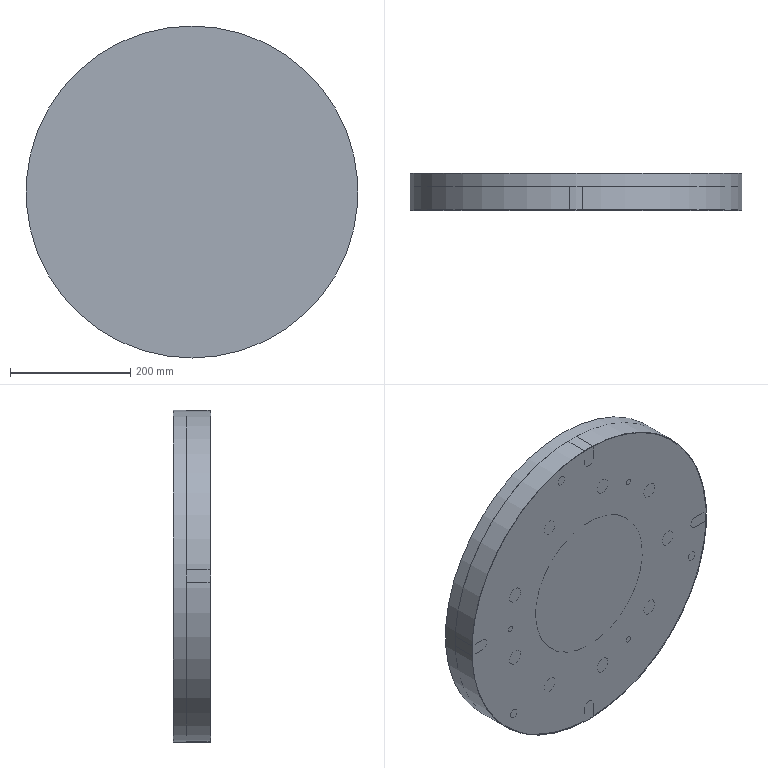NC program | NX | posted with a generic post | part box 552 x 62 x 552 mm
Whole program:
N10 G17 G21 G94 G90
(CAVITY_MILL_1 , TOOL : D8)
N12 T03 M6
N14 G54
N16 G17 G0 G90 X136.011 Y-125.254 S900 M3
N18 G43 Z19. H3
N20 Z-6.5
N22 G94 G1 X136.461 Y-125.633 Z-6.521 F80.
N24 X137.059 Y-126.025 Z-6.546
N26 X147.91 Y-113.092 Z-7.135
N28 X147.421 Y-112.572 Z-7.16
N30 X146.976 Y-112.198 Z-7.18
N32 X146.378 Y-111.807 Z-7.205
N34 X140.952 Y-118.273 Z-7.5
N36 X135.526 Y-124.739
N38 G3 X137.059 Y-126.025 R8.5
N40 G1 X147.91 Y-113.092
N42 G3 X146.378 Y-111.807 R8.49
N44 G1 X140.952 Y-118.273
N46 G3 X141.014 Y-118.977 R0.5
N48 X141.718 Y-118.916 R0.5
N50 G1 Z-7.3
N52 G0 Z-6.7
N54 X136.011 Y-125.254
N56 Z-7.
N58 G1 X136.461 Y-125.633 Z-7.021
N60 X137.059 Y-126.025 Z-7.046
N62 X147.91 Y-113.092 Z-7.635
N64 X147.421 Y-112.572 Z-7.66
N66 X146.976 Y-112.198 Z-7.68
N68 X146.378 Y-111.807 Z-7.705
N70 X140.952 Y-118.273 Z-8.
N72 X135.526 Y-124.739
N74 G3 X137.059 Y-126.025 R8.5
N76 G1 X147.91 Y-113.092
N78 G3 X146.378 Y-111.807 R8.49
N80 G1 X140.952 Y-118.273
N82 G3 X141.014 Y-118.977 R0.5
N84 X141.718 Y-118.916 R0.5
N86 G1 Z-7.8
N88 G0 Z-6.7
N90 X136.011 Y-125.254
N92 Z-7.5
N94 G1 X136.461 Y-125.633 Z-7.521
N96 X137.059 Y-126.025 Z-7.546
N98 X147.91 Y-113.092 Z-8.135
N100 X147.421 Y-112.572 Z-8.16
N102 X146.976 Y-112.198 Z-8.18
N104 X146.378 Y-111.807 Z-8.205
N106 X140.952 Y-118.273 Z-8.5
N108 X135.526 Y-124.739
N110 G3 X137.059 Y-126.025 R8.5
N112 G1 X147.91 Y-113.092
N114 G3 X146.378 Y-111.807 R8.49
N116 G1 X140.952 Y-118.273
N118 G3 X141.014 Y-118.977 R0.5
N120 X141.718 Y-118.916 R0.5
N122 G1 Z-8.3
N124 G0 Z-6.7
N126 X136.011 Y-125.254
N128 Z-8.
N130 G1 X136.461 Y-125.633 Z-8.021
N132 X137.059 Y-126.025 Z-8.046
N134 X147.91 Y-113.092 Z-8.635
N136 X147.421 Y-112.572 Z-8.66
N138 X146.976 Y-112.198 Z-8.68
N140 X146.378 Y-111.807 Z-8.705
N142 X140.952 Y-118.273 Z-9.
N144 X135.526 Y-124.739
N146 G3 X137.059 Y-126.025 R8.5
N148 G1 X147.91 Y-113.092
N150 G3 X146.378 Y-111.807 R8.49
N152 G1 X140.952 Y-118.273
N154 G3 X141.014 Y-118.977 R0.5
N156 X141.718 Y-118.916 R0.5
N158 G1 Z-8.8
N160 G0 Z-6.7
N162 X136.011 Y-125.254
N164 Z-8.5
N166 G1 X136.461 Y-125.633 Z-8.521
N168 X137.059 Y-126.025 Z-8.546
N170 X147.91 Y-113.092 Z-9.135
N172 X147.421 Y-112.572 Z-9.16
N174 X146.976 Y-112.198 Z-9.18
N176 X146.378 Y-111.807 Z-9.205
N178 X140.952 Y-118.273 Z-9.5
N180 X135.526 Y-124.739
N182 G3 X137.059 Y-126.025 R8.5
N184 G1 X147.91 Y-113.092
N186 G3 X146.378 Y-111.807 R8.49
N188 G1 X140.952 Y-118.273
N190 G3 X141.014 Y-118.977 R0.5
N192 X141.718 Y-118.916 R0.5
N194 G1 Z-9.3
N196 G0 Z-6.7
N198 X136.011 Y-125.254
N200 Z-9.
N202 G1 X136.461 Y-125.633 Z-9.021
N204 X137.059 Y-126.025 Z-9.046
N206 X147.91 Y-113.092 Z-9.635
N208 X147.421 Y-112.572 Z-9.66
N210 X146.976 Y-112.198 Z-9.68
N212 X146.378 Y-111.807 Z-9.705
N214 X140.952 Y-118.273 Z-10.
N216 X135.526 Y-124.739
N218 G3 X137.059 Y-126.025 R8.5
N220 G1 X147.91 Y-113.092
N222 G3 X146.378 Y-111.807 R8.49
N224 G1 X140.952 Y-118.273
N226 G3 X141.014 Y-118.977 R0.5
N228 X141.718 Y-118.916 R0.5
N230 G1 Z-9.8
N232 G0 Z-6.7
N234 X136.011 Y-125.254
N236 Z-9.5
N238 G1 X136.461 Y-125.633 Z-9.521
N240 X137.059 Y-126.025 Z-9.546
N242 X147.91 Y-113.092 Z-10.135
N244 X147.421 Y-112.572 Z-10.16
N246 X146.976 Y-112.198 Z-10.18
N248 X146.378 Y-111.807 Z-10.205
N250 X140.952 Y-118.273 Z-10.5
N252 X135.526 Y-124.739
N254 G3 X137.059 Y-126.025 R8.5
N256 G1 X147.91 Y-113.092
N258 G3 X146.378 Y-111.807 R8.49
N260 G1 X140.952 Y-118.273
N262 G3 X141.014 Y-118.977 R0.5
N264 X141.718 Y-118.916 R0.5
N266 G1 Z-10.3
N268 G0 Z-6.7
N270 X136.011 Y-125.254
N272 Z-10.
N274 G1 X136.461 Y-125.633 Z-10.021
N276 X137.059 Y-126.025 Z-10.046
N278 X147.91 Y-113.092 Z-10.635
N280 X147.421 Y-112.572 Z-10.66
N282 X146.976 Y-112.198 Z-10.68
N284 X146.378 Y-111.807 Z-10.705
N286 X140.952 Y-118.273 Z-11.
N288 X135.526 Y-124.739
N290 G3 X137.059 Y-126.025 R8.5
N292 G1 X147.91 Y-113.092
N294 G3 X146.378 Y-111.807 R8.49
N296 G1 X140.952 Y-118.273
N298 G3 X141.014 Y-118.977 R0.5
N300 X141.718 Y-118.916 R0.5
N302 G1 Z-10.8
N304 G0 Z-6.7
N306 X136.011 Y-125.254
N308 Z-10.5
N310 G1 X136.461 Y-125.633 Z-10.521
N312 X137.059 Y-126.025 Z-10.546
N314 X147.91 Y-113.092 Z-11.135
N316 X147.421 Y-112.572 Z-11.16
N318 X146.976 Y-112.198 Z-11.18
N320 X146.378 Y-111.807 Z-11.205
N322 X140.952 Y-118.273 Z-11.5
N324 X135.526 Y-124.739
N326 G3 X137.059 Y-126.025 R8.5
N328 G1 X147.91 Y-113.092
N330 G3 X146.378 Y-111.807 R8.49
N332 G1 X140.952 Y-118.273
N334 G3 X141.014 Y-118.977 R0.5
N336 X141.718 Y-118.916 R0.5
N338 G1 Z-11.3
N340 G0 Z-6.7
N342 X136.011 Y-125.254
N344 Z-11.
N346 G1 X136.461 Y-125.633 Z-11.021
N348 X137.059 Y-126.025 Z-11.046
N350 X147.91 Y-113.092 Z-11.635
N352 X147.421 Y-112.572 Z-11.66
N354 X146.976 Y-112.198 Z-11.68
N356 X146.378 Y-111.807 Z-11.705
N358 X140.952 Y-118.273 Z-12.
N360 X135.526 Y-124.739
N362 G3 X137.059 Y-126.025 R8.5
N364 G1 X147.91 Y-113.092
N366 G3 X146.378 Y-111.807 R8.49
N368 G1 X140.952 Y-118.273
N370 G3 X141.014 Y-118.977 R0.5
N372 X141.718 Y-118.916 R0.5
N374 G1 Z-11.8
N376 G0 Z-6.7
N378 X136.011 Y-125.254
N380 Z-11.5
N382 G1 X136.461 Y-125.633 Z-11.521
N384 X137.059 Y-126.025 Z-11.546
N386 X147.91 Y-113.092 Z-12.135
N388 X147.421 Y-112.572 Z-12.16
N390 X146.976 Y-112.198 Z-12.18
N392 X146.378 Y-111.807 Z-12.205
N394 X140.952 Y-118.273 Z-12.5
N396 X135.526 Y-124.739
N398 G3 X137.059 Y-126.025 R8.5
N400 G1 X147.91 Y-113.092
N402 G3 X146.378 Y-111.807 R8.49
N404 G1 X140.952 Y-118.273
N406 G3 X141.014 Y-118.977 R0.5
N408 X141.718 Y-118.916 R0.5
N410 G1 Z-12.3
N412 G0 Z-6.7
N414 X136.011 Y-125.254
N416 Z-12.
N418 G1 X136.461 Y-125.633 Z-12.021
N420 X137.059 Y-126.025 Z-12.046
N422 X147.91 Y-113.092 Z-12.635
N424 X147.421 Y-112.572 Z-12.66
N426 X146.976 Y-112.198 Z-12.68
N428 X146.378 Y-111.807 Z-12.705
N430 X140.952 Y-118.273 Z-13.
N432 X135.526 Y-124.739
N434 G3 X137.059 Y-126.025 R8.5
N436 G1 X147.91 Y-113.092
N438 G3 X146.378 Y-111.807 R8.49
N440 G1 X140.952 Y-118.273
N442 G3 X141.014 Y-118.977 R0.5
N444 X141.718 Y-118.916 R0.5
N446 G1 Z-12.8
N448 G0 Z-6.7
N450 X136.011 Y-125.254
N452 Z-12.5
N454 G1 X136.461 Y-125.633 Z-12.521
N456 X137.059 Y-126.025 Z-12.546
N458 X147.91 Y-113.092 Z-13.135
N460 X147.421 Y-112.572 Z-13.16
N462 X146.976 Y-112.198 Z-13.18
N464 X146.378 Y-111.807 Z-13.205
N466 X140.952 Y-118.273 Z-13.5
N468 X135.526 Y-124.739
N470 G3 X137.059 Y-126.025 R8.5
N472 G1 X147.91 Y-113.092
N474 G3 X146.378 Y-111.807 R8.49
N476 G1 X140.952 Y-118.273
N478 G3 X141.014 Y-118.977 R0.5
N480 X141.718 Y-118.916 R0.5
N482 G1 Z-13.3
N484 G0 Z-6.7
N486 X136.011 Y-125.254
N488 Z-13.
N490 G1 X136.461 Y-125.633 Z-13.021
N492 X137.059 Y-126.025 Z-13.046
N494 X147.91 Y-113.092 Z-13.635
N496 X147.421 Y-112.572 Z-13.66
N498 X146.976 Y-112.198 Z-13.68
N500 X146.378 Y-111.807 Z-13.705
N502 X140.952 Y-118.273 Z-14.
N504 X135.526 Y-124.739
N506 G3 X137.059 Y-126.025 R8.5
N508 G1 X147.91 Y-113.092
N510 G3 X146.378 Y-111.807 R8.49
N512 G1 X140.952 Y-118.273
N514 G3 X141.014 Y-118.977 R0.5
N516 X141.718 Y-118.916 R0.5
N518 G1 Z-13.8
N520 G0 Z-6.7
N522 X136.011 Y-125.254
N524 Z-13.5
N526 G1 X136.461 Y-125.633 Z-13.521
N528 X137.059 Y-126.025 Z-13.546
N530 X147.91 Y-113.092 Z-14.135
N532 X147.421 Y-112.572 Z-14.16
N534 X146.976 Y-112.198 Z-14.18
N536 X146.378 Y-111.807 Z-14.205
N538 X140.952 Y-118.273 Z-14.5
N540 X135.526 Y-124.739
N542 G3 X137.059 Y-126.025 R8.5
N544 G1 X147.91 Y-113.092
N546 G3 X146.378 Y-111.807 R8.49
N548 G1 X140.952 Y-118.273
N550 G3 X141.014 Y-118.977 R0.5
N552 X141.718 Y-118.916 R0.5
N554 G1 Z-14.3
N556 G0 Z-6.7
N558 X136.011 Y-125.254
N560 Z-14.
N562 G1 X136.461 Y-125.633 Z-14.021
N564 X137.059 Y-126.025 Z-14.046
N566 X147.91 Y-113.092 Z-14.635
N568 X147.421 Y-112.572 Z-14.66
N570 X146.976 Y-112.198 Z-14.68
N572 X146.378 Y-111.807 Z-14.705
N574 X140.952 Y-118.273 Z-15.
N576 X135.526 Y-124.739
N578 G3 X137.059 Y-126.025 R8.5
N580 G1 X147.91 Y-113.092
N582 G3 X146.378 Y-111.807 R8.49
N584 G1 X140.952 Y-118.273
N586 G3 X141.014 Y-118.977 R0.5
N588 X141.718 Y-118.916 R0.5
N590 G1 Z-14.8
N592 G0 Z-6.7
N594 X136.011 Y-125.254
N596 Z-14.5
N598 G1 X136.461 Y-125.633 Z-14.521
N600 X137.059 Y-126.025 Z-14.546
N602 X147.91 Y-113.092 Z-15.135
N604 X147.421 Y-112.572 Z-15.16
N606 X146.976 Y-112.198 Z-15.18
N608 X146.378 Y-111.807 Z-15.205
N610 X140.952 Y-118.273 Z-15.5
N612 X135.526 Y-124.739
N614 G3 X137.059 Y-126.025 R8.5
N616 G1 X147.91 Y-113.092
N618 G3 X146.378 Y-111.807 R8.49
N620 G1 X140.952 Y-118.273
N622 G3 X141.014 Y-118.977 R0.5
N624 X141.718 Y-118.916 R0.5
N626 G1 Z-15.3
N628 G0 Z-6.7
N630 X136.011 Y-125.254
N632 Z-15.
N634 G1 X136.461 Y-125.633 Z-15.021
N636 X137.059 Y-126.025 Z-15.046
N638 X147.91 Y-113.092 Z-15.635
N640 X147.421 Y-112.572 Z-15.66
N642 X146.976 Y-112.198 Z-15.68
N644 X146.378 Y-111.807 Z-15.705
N646 X140.952 Y-118.273 Z-16.
N648 X135.526 Y-124.739
N650 G3 X137.059 Y-126.025 R8.5
N652 G1 X147.91 Y-113.092
N654 G3 X146.378 Y-111.807 R8.49
N656 G1 X140.952 Y-118.273
N658 G3 X141.014 Y-118.977 R0.5
N660 X141.718 Y-118.916 R0.5
N662 G1 Z-15.8
N664 G0 Z-6.7
N666 X136.011 Y-125.254
N668 Z-15.5
N670 G1 X136.461 Y-125.633 Z-15.521
N672 X137.059 Y-126.025 Z-15.546
N674 X147.91 Y-113.092 Z-16.135
N676 X147.421 Y-112.572 Z-16.16
N678 X146.976 Y-112.198 Z-16.18
N680 X146.378 Y-111.807 Z-16.205
N682 X140.952 Y-118.273 Z-16.5
N684 X135.526 Y-124.739
N686 G3 X137.059 Y-126.025 R8.5
N688 G1 X147.91 Y-113.092
N690 G3 X146.378 Y-111.807 R8.49
N692 G1 X140.952 Y-118.273
N694 G3 X141.014 Y-118.977 R0.5
N696 X141.718 Y-118.916 R0.5
N698 G1 Z-16.3
N700 G0 Z-6.7
N702 X136.011 Y-125.254
N704 Z-16.
N706 G1 X136.461 Y-125.633 Z-16.021
N708 X137.059 Y-126.025 Z-16.046
N710 X147.91 Y-113.092 Z-16.635
N712 X147.421 Y-112.572 Z-16.66
N714 X146.976 Y-112.198 Z-16.68
N716 X146.378 Y-111.807 Z-16.705
N718 X140.952 Y-118.273 Z-17.
N720 X135.526 Y-124.739
N722 G3 X137.059 Y-126.025 R8.5
N724 G1 X147.91 Y-113.092
N726 G3 X146.378 Y-111.807 R8.49
N728 G1 X140.952 Y-118.273
N730 G3 X141.014 Y-118.977 R0.5
N732 X141.718 Y-118.916 R0.5
N734 G1 Z-16.8
N736 G0 Z-6.7
N738 X136.011 Y-125.254
N740 Z-16.5
N742 G1 X136.461 Y-125.633 Z-16.521
N744 X137.059 Y-126.025 Z-16.546
N746 X147.91 Y-113.092 Z-17.135
N748 X147.421 Y-112.572 Z-17.16
N750 X146.976 Y-112.198 Z-17.18
N752 X146.378 Y-111.807 Z-17.205
N754 X140.952 Y-118.273 Z-17.5
N756 X135.526 Y-124.739
N758 G3 X137.059 Y-126.025 R8.5
N760 G1 X147.91 Y-113.092
N762 G3 X146.378 Y-111.807 R8.49
N764 G1 X140.952 Y-118.273
N766 G3 X141.014 Y-118.977 R0.5
N768 X141.718 Y-118.916 R0.5
N770 G1 Z-17.3
N772 G0 Z-6.7
N774 X136.011 Y-125.254
N776 Z-17.
N778 G1 X136.461 Y-125.633 Z-17.021
N780 X137.059 Y-126.025 Z-17.046
N782 X147.91 Y-113.092 Z-17.635
N784 X147.421 Y-112.572 Z-17.66
N786 X146.976 Y-112.198 Z-17.68
N788 X146.378 Y-111.807 Z-17.705
N790 X140.952 Y-118.273 Z-18.
N792 X135.526 Y-124.739
N794 G3 X137.059 Y-126.025 R8.5
N796 G1 X147.91 Y-113.092
N798 G3 X146.378 Y-111.807 R8.49
N800 G1 X140.952 Y-118.273
N802 G3 X141.014 Y-118.977 R0.5
N804 X141.718 Y-118.916 R0.5
N806 G1 Z-17.8
N808 G0 Z-6.7
N810 X136.011 Y-125.254
N812 Z-17.5
N814 G1 X136.461 Y-125.633 Z-17.521
N816 X137.059 Y-126.025 Z-17.546
N818 X147.91 Y-113.092 Z-18.135
N820 X147.421 Y-112.572 Z-18.16
N822 X146.976 Y-112.198 Z-18.18
N824 X146.378 Y-111.807 Z-18.205
N826 X140.952 Y-118.273 Z-18.5
N828 X135.526 Y-124.739
N830 G3 X137.059 Y-126.025 R8.5
N832 G1 X147.91 Y-113.092
N834 G3 X146.378 Y-111.807 R8.49
N836 G1 X140.952 Y-118.273
N838 G3 X141.014 Y-118.977 R0.5
N840 X141.718 Y-118.916 R0.5
N842 G1 Z-18.3
N844 G0 Z-6.7
N846 X136.011 Y-125.254
N848 Z-18.
N850 G1 X136.461 Y-125.633 Z-18.021
N852 X137.059 Y-126.025 Z-18.046
N854 X147.91 Y-113.092 Z-18.635
N856 X147.421 Y-112.572 Z-18.66
N858 X146.976 Y-112.198 Z-18.68
N860 X146.378 Y-111.807 Z-18.705
N862 X140.952 Y-118.273 Z-19.
N864 X135.526 Y-124.739
N866 G3 X137.059 Y-126.025 R8.5
N868 G1 X147.91 Y-113.092
N870 G3 X146.378 Y-111.807 R8.49
N872 G1 X140.952 Y-118.273
N874 G3 X141.014 Y-118.977 R0.5
N876 X141.718 Y-118.916 R0.5
N878 G1 Z-18.8
N880 G0 Z-6.7
N882 X136.011 Y-125.254
N884 Z-18.5
N886 G1 X136.461 Y-125.633 Z-18.521
N888 X137.059 Y-126.025 Z-18.546
N890 X147.91 Y-113.092 Z-19.135
N892 X147.421 Y-112.572 Z-19.16
N894 X146.976 Y-112.198 Z-19.18
N896 X146.378 Y-111.807 Z-19.205
N898 X140.952 Y-118.273 Z-19.5
N900 X135.526 Y-124.739
N902 G3 X137.059 Y-126.025 R8.5
N904 G1 X147.91 Y-113.092
N906 G3 X146.378 Y-111.807 R8.49
N908 G1 X140.952 Y-118.273
N910 G3 X141.014 Y-118.977 R0.5
N912 X141.718 Y-118.916 R0.5
N914 G1 Z-19.3
N916 G0 Z-6.7
N918 X136.011 Y-125.254
N920 Z-19.
N922 G1 X136.461 Y-125.633 Z-19.021
N924 X137.059 Y-126.025 Z-19.046
N926 X147.91 Y-113.092 Z-19.635
N928 X147.421 Y-112.572 Z-19.66
N930 X146.976 Y-112.198 Z-19.68
N932 X146.378 Y-111.807 Z-19.705
N934 X140.952 Y-118.273 Z-20.
N936 X135.526 Y-124.739
N938 G3 X137.059 Y-126.025 R8.5
N940 G1 X147.91 Y-113.092
N942 G3 X146.378 Y-111.807 R8.49
N944 G1 X140.952 Y-118.273
N946 G3 X141.014 Y-118.977 R0.5
N948 X141.718 Y-118.916 R0.5
N950 G1 Z-19.8
N952 G0 Z-6.7
N954 X136.011 Y-125.254
N956 Z-19.5
N958 G1 X136.461 Y-125.633 Z-19.521
N960 X137.059 Y-126.025 Z-19.546
N962 X147.91 Y-113.092 Z-20.135
N964 X147.421 Y-112.572 Z-20.16
N966 X146.976 Y-112.198 Z-20.18
N968 X146.378 Y-111.807 Z-20.205
N970 X140.952 Y-118.273 Z-20.5
N972 X135.526 Y-124.739
N974 G3 X137.059 Y-126.025 R8.5
N976 G1 X147.91 Y-113.092
N978 G3 X146.378 Y-111.807 R8.49
N980 G1 X140.952 Y-118.273
N982 G3 X141.014 Y-118.977 R0.5
N984 X141.718 Y-118.916 R0.5
N986 G1 Z-20.3
N988 G0 Z-6.7
N990 X136.011 Y-125.254
N992 Z-20.
N994 G1 X136.461 Y-125.633 Z-20.021
N996 X137.059 Y-126.025 Z-20.046
N998 X147.91 Y-113.092 Z-20.635
N1000 X147.421 Y-112.572 Z-20.66
N1002 X146.976 Y-112.198 Z-20.68
N1004 X146.378 Y-111.807 Z-20.705
N1006 X140.952 Y-118.273 Z-21.
N1008 X135.526 Y-124.739
N1010 G3 X137.059 Y-126.025 R8.5
N1012 G1 X147.91 Y-113.092
N1014 G3 X146.378 Y-111.807 R8.49
N1016 G1 X140.952 Y-118.273
N1018 G3 X141.014 Y-118.977 R0.5
N1020 X141.718 Y-118.916 R0.5
N1022 G1 Z-20.8
N1024 G0 Z-6.7
N1026 X136.011 Y-125.254
N1028 Z-20.5
N1030 G1 X136.461 Y-125.633 Z-20.521
N1032 X137.059 Y-126.025 Z-20.546
N1034 X147.91 Y-113.092 Z-21.135
N1036 X147.421 Y-112.572 Z-21.16
N1038 X146.976 Y-112.198 Z-21.18
N1040 X146.378 Y-111.807 Z-21.205
N1042 X140.952 Y-118.273 Z-21.5
N1044 X135.526 Y-124.739
N1046 G3 X137.059 Y-126.025 R8.5
N1048 G1 X147.91 Y-113.092
N1050 G3 X146.378 Y-111.807 R8.49
N1052 G1 X140.952 Y-118.273
N1054 G3 X141.014 Y-118.977 R0.5
N1056 X141.718 Y-118.916 R0.5
N1058 G1 Z-21.3
N1060 G0 Z-6.7
N1062 X136.011 Y-125.254
N1064 Z-21.
N1066 G1 X136.461 Y-125.633 Z-21.021
N1068 X137.059 Y-126.025 Z-21.046
N1070 X147.91 Y-113.092 Z-21.635
N1072 X147.421 Y-112.572 Z-21.66
N1074 X146.976 Y-112.198 Z-21.68
N1076 X146.378 Y-111.807 Z-21.705
N1078 X140.952 Y-118.273 Z-22.
N1080 X135.526 Y-124.739
N1082 G3 X137.059 Y-126.025 R8.5
N1084 G1 X147.91 Y-113.092
N1086 G3 X146.378 Y-111.807 R8.49
N1088 G1 X140.952 Y-118.273
N1090 G3 X141.014 Y-118.977 R0.5
N1092 X141.718 Y-118.916 R0.5
N1094 G1 Z-21.8
N1096 G0 Z-6.7
N1098 X136.011 Y-125.254
N1100 Z-21.5
N1102 G1 X136.461 Y-125.633 Z-21.521
N1104 X137.059 Y-126.025 Z-21.546
N1106 X147.91 Y-113.092 Z-22.135
N1108 X147.421 Y-112.572 Z-22.16
N1110 X146.976 Y-112.198 Z-22.18
N1112 X146.378 Y-111.807 Z-22.205
N1114 X140.952 Y-118.273 Z-22.5
N1116 X135.526 Y-124.739
N1118 G3 X137.059 Y-126.025 R8.5
N1120 G1 X147.91 Y-113.092
N1122 G3 X146.378 Y-111.807 R8.49
N1124 G1 X140.952 Y-118.273
N1126 G3 X141.014 Y-118.977 R0.5
N1128 X141.718 Y-118.916 R0.5
N1130 G1 Z-22.3
N1132 G0 Z-6.7
N1134 X136.011 Y-125.254
N1136 Z-22.
N1138 G1 X136.461 Y-125.633 Z-22.021
N1140 X137.059 Y-126.025 Z-22.046
N1142 X147.91 Y-113.092 Z-22.635
N1144 X147.421 Y-112.572 Z-22.66
N1146 X146.976 Y-112.198 Z-22.68
N1148 X146.378 Y-111.807 Z-22.705
N1150 X140.952 Y-118.273 Z-23.
N1152 X135.526 Y-124.739
N1154 G3 X137.059 Y-126.025 R8.5
N1156 G1 X147.91 Y-113.092
N1158 G3 X146.378 Y-111.807 R8.49
N1160 G1 X140.952 Y-118.273
N1162 G3 X141.014 Y-118.977 R0.5
N1164 X141.718 Y-118.916 R0.5
N1166 G1 Z-22.8
N1168 G0 Z-6.7
N1170 X136.011 Y-125.254
N1172 Z-22.5
N1174 G1 X136.461 Y-125.633 Z-22.521
N1176 X137.059 Y-126.025 Z-22.546
N1178 X147.91 Y-113.092 Z-23.135
N1180 X147.421 Y-112.572 Z-23.16
N1182 X146.976 Y-112.198 Z-23.18
N1184 X146.378 Y-111.807 Z-23.205
N1186 X140.952 Y-118.273 Z-23.5
N1188 X135.526 Y-124.739
N1190 G3 X137.059 Y-126.025 R8.5
N1192 G1 X147.91 Y-113.092
N1194 G3 X146.378 Y-111.807 R8.49
N1196 G1 X140.952 Y-118.273
N1198 G3 X141.014 Y-118.977 R0.5
N1200 X141.718 Y-118.916 R0.5
N1202 G1 Z-23.3
N1204 G0 Z-6.7
N1206 X136.011 Y-125.254
N1208 Z-23.
N1210 G1 X136.461 Y-125.633 Z-23.021
N1212 X137.059 Y-126.025 Z-23.046
N1214 X147.91 Y-113.092 Z-23.635
N1216 X147.421 Y-112.572 Z-23.66
N1218 X146.976 Y-112.198 Z-23.68
N1220 X146.378 Y-111.807 Z-23.705
N1222 X140.952 Y-118.273 Z-24.
N1224 X135.526 Y-124.739
N1226 G3 X137.059 Y-126.025 R8.5
N1228 G1 X147.91 Y-113.092
N1230 G3 X146.378 Y-111.807 R8.49
N1232 G1 X140.952 Y-118.273
N1234 G3 X141.014 Y-118.977 R0.5
N1236 X141.718 Y-118.916 R0.5
N1238 G1 Z-23.8
N1240 G0 Z-6.7
N1242 X136.011 Y-125.254
N1244 Z-23.5
N1246 G1 X136.461 Y-125.633 Z-23.521
N1248 X137.059 Y-126.025 Z-23.546
N1250 X147.91 Y-113.092 Z-24.135
N1252 X147.421 Y-112.572 Z-24.16
N1254 X146.976 Y-112.198 Z-24.18
N1256 X146.378 Y-111.807 Z-24.205
N1258 X140.952 Y-118.273 Z-24.5
N1260 X135.526 Y-124.739
N1262 G3 X137.059 Y-126.025 R8.5
N1264 G1 X147.91 Y-113.092
N1266 G3 X146.378 Y-111.807 R8.49
N1268 G1 X140.952 Y-118.273
N1270 G3 X141.014 Y-118.977 R0.5
N1272 X141.718 Y-118.916 R0.5
N1274 G1 Z-24.3
N1276 G0 Z-6.7
N1278 X136.011 Y-125.254
N1280 Z-24.
N1282 G1 X136.461 Y-125.633 Z-24.021
N1284 X137.059 Y-126.025 Z-24.046
N1286 X147.91 Y-113.092 Z-24.635
N1288 X147.421 Y-112.572 Z-24.66
N1290 X146.976 Y-112.198 Z-24.68
N1292 X146.378 Y-111.807 Z-24.705
N1294 X140.952 Y-118.273 Z-25.
N1296 X135.526 Y-124.739
N1298 G3 X137.059 Y-126.025 R8.5
N1300 G1 X147.91 Y-113.092
N1302 G3 X146.378 Y-111.807 R8.49
N1304 G1 X140.952 Y-118.273
N1306 G3 X141.014 Y-118.977 R0.5
N1308 X141.718 Y-118.916 R0.5
N1310 G1 Z-24.8
N1312 G0 Z-6.7
N1314 X136.011 Y-125.254
N1316 Z-24.5
N1318 G1 X136.461 Y-125.633 Z-24.521
N1320 X137.059 Y-126.025 Z-24.546
N1322 X147.91 Y-113.092 Z-25.135
N1324 X147.421 Y-112.572 Z-25.16
N1326 X146.976 Y-112.198 Z-25.18
N1328 X146.378 Y-111.807 Z-25.205
N1330 X140.952 Y-118.273 Z-25.5
N1332 X135.526 Y-124.739
N1334 G3 X137.059 Y-126.025 R8.5
N1336 G1 X147.91 Y-113.092
N1338 G3 X146.378 Y-111.807 R8.49
N1340 G1 X140.952 Y-118.273
N1342 G3 X141.014 Y-118.977 R0.5
N1344 X141.718 Y-118.916 R0.5
N1346 G1 Z-25.3
N1348 G0 Z-6.7
N1350 X136.011 Y-125.254
N1352 Z-25.
N1354 G1 X136.461 Y-125.633 Z-25.021
N1356 X137.059 Y-126.025 Z-25.046
N1358 X147.91 Y-113.092 Z-25.635
N1360 X147.421 Y-112.572 Z-25.66
N1362 X146.976 Y-112.198 Z-25.68
N1364 X146.378 Y-111.807 Z-25.705
N1366 X140.952 Y-118.273 Z-26.
N1368 X135.526 Y-124.739
N1370 G3 X137.059 Y-126.025 R8.5
N1372 G1 X147.91 Y-113.092
N1374 G3 X146.378 Y-111.807 R8.49
N1376 G1 X140.952 Y-118.273
N1378 G3 X141.014 Y-118.977 R0.5
N1380 X141.718 Y-118.916 R0.5
N1382 G1 Z-25.8
N1384 G0 Z-6.7
N1386 X136.011 Y-125.254
N1388 Z-25.5
N1390 G1 X136.461 Y-125.633 Z-25.521
N1392 X137.059 Y-126.025 Z-25.546
N1394 X147.91 Y-113.092 Z-26.135
N1396 X147.421 Y-112.572 Z-26.16
N1398 X146.976 Y-112.198 Z-26.18
N1400 X146.378 Y-111.807 Z-26.205
N1402 X140.952 Y-118.273 Z-26.5
N1404 X135.526 Y-124.739
N1406 G3 X137.059 Y-126.025 R8.5
N1408 G1 X147.91 Y-113.092
N1410 G3 X146.378 Y-111.807 R8.49
N1412 G1 X140.952 Y-118.273
N1414 G3 X141.014 Y-118.977 R0.5
N1416 X141.718 Y-118.916 R0.5
N1418 G1 Z-26.3
N1420 G0 Z-6.7
N1422 X136.011 Y-125.254
N1424 Z-26.
N1426 G1 X136.461 Y-125.633 Z-26.021
N1428 X137.059 Y-126.025 Z-26.046
N1430 X147.91 Y-113.092 Z-26.635
N1432 X147.421 Y-112.572 Z-26.66
N1434 X146.976 Y-112.198 Z-26.68
N1436 X146.378 Y-111.807 Z-26.705
N1438 X140.952 Y-118.273 Z-27.
N1440 X135.526 Y-124.739
N1442 G3 X137.059 Y-126.025 R8.5
N1444 G1 X147.91 Y-113.092
N1446 G3 X146.378 Y-111.807 R8.49
N1448 G1 X140.952 Y-118.273
N1450 G3 X141.014 Y-118.977 R0.5
N1452 X141.718 Y-118.916 R0.5
N1454 G1 Z-26.8
N1456 G0 Z-6.7
N1458 X136.011 Y-125.254
N1460 Z-26.5
N1462 G1 X136.461 Y-125.633 Z-26.521
N1464 X137.059 Y-126.025 Z-26.546
N1466 X147.91 Y-113.092 Z-27.135
N1468 X147.421 Y-112.572 Z-27.16
N1470 X146.976 Y-112.198 Z-27.18
N1472 X146.378 Y-111.807 Z-27.205
N1474 X140.952 Y-118.273 Z-27.5
N1476 X135.526 Y-124.739
N1478 G3 X137.059 Y-126.025 R8.5
N1480 G1 X147.91 Y-113.092
N1482 G3 X146.378 Y-111.807 R8.49
N1484 G1 X140.952 Y-118.273
N1486 G3 X141.014 Y-118.977 R0.5
N1488 X141.718 Y-118.916 R0.5
N1490 G1 Z-27.3
N1492 G0 Z-6.7
N1494 X136.011 Y-125.254
N1496 Z-27.
N1498 G1 X136.461 Y-125.633 Z-27.021
N1500 X137.059 Y-126.025 Z-27.046
N1502 X147.91 Y-113.092 Z-27.635
N1504 X147.421 Y-112.572 Z-27.66
N1506 X146.976 Y-112.198 Z-27.68
N1508 X146.378 Y-111.807 Z-27.705
N1510 X140.952 Y-118.273 Z-28.
N1512 X135.526 Y-124.739
N1514 G3 X137.059 Y-126.025 R8.5
N1516 G1 X147.91 Y-113.092
N1518 G3 X146.378 Y-111.807 R8.49
N1520 G1 X140.952 Y-118.273
N1522 G3 X141.014 Y-118.977 R0.5
N1524 X141.718 Y-118.916 R0.5
N1526 G1 Z-27.8
N1528 G0 Z-6.7
N1530 X136.011 Y-125.254
N1532 Z-27.5
N1534 G1 X136.461 Y-125.633 Z-27.521
N1536 X137.059 Y-126.025 Z-27.546
N1538 X147.91 Y-113.092 Z-28.135
N1540 X147.421 Y-112.572 Z-28.16
N1542 X146.976 Y-112.198 Z-28.18
N1544 X146.378 Y-111.807 Z-28.205
N1546 X140.952 Y-118.273 Z-28.5
N1548 X135.526 Y-124.739
N1550 G3 X137.059 Y-126.025 R8.5
N1552 G1 X147.91 Y-113.092
N1554 G3 X146.378 Y-111.807 R8.49
N1556 G1 X140.952 Y-118.273
N1558 G3 X141.014 Y-118.977 R0.5
N1560 X141.718 Y-118.916 R0.5
N1562 G1 Z-28.3
N1564 G0 Z-6.7
N1566 X136.011 Y-125.254
N1568 Z-28.
N1570 G1 X136.461 Y-125.633 Z-28.021
N1572 X137.059 Y-126.025 Z-28.046
N1574 X147.91 Y-113.092 Z-28.635
N1576 X147.421 Y-112.572 Z-28.66
N1578 X146.976 Y-112.198 Z-28.68
N1580 X146.378 Y-111.807 Z-28.705
N1582 X140.952 Y-118.273 Z-29.
N1584 X135.526 Y-124.739
N1586 G3 X137.059 Y-126.025 R8.5
N1588 G1 X147.91 Y-113.092
N1590 G3 X146.378 Y-111.807 R8.49
N1592 G1 X140.952 Y-118.273
N1594 G3 X141.014 Y-118.977 R0.5
N1596 X141.718 Y-118.916 R0.5
N1598 G1 Z-28.8
N1600 G0 Z-6.7
N1602 X136.011 Y-125.254
N1604 Z-28.5
N1606 G1 X136.461 Y-125.633 Z-28.521
N1608 X137.059 Y-126.025 Z-28.546
N1610 X147.91 Y-113.092 Z-29.135
N1612 X147.421 Y-112.572 Z-29.16
N1614 X146.976 Y-112.198 Z-29.18
N1616 X146.378 Y-111.807 Z-29.205
N1618 X140.952 Y-118.273 Z-29.5
N1620 X135.526 Y-124.739
N1622 G3 X137.059 Y-126.025 R8.5
N1624 G1 X147.91 Y-113.092
N1626 G3 X146.378 Y-111.807 R8.49
N1628 G1 X140.952 Y-118.273
N1630 G3 X141.014 Y-118.977 R0.5
N1632 X141.718 Y-118.916 R0.5
N1634 G1 Z-29.3
N1636 G0 Z-6.7
N1638 X136.011 Y-125.254
N1640 Z-29.
N1642 G1 X136.461 Y-125.633 Z-29.021
N1644 X137.059 Y-126.025 Z-29.046
N1646 X147.91 Y-113.092 Z-29.635
N1648 X147.42 Y-112.572 Z-29.66
N1650 X146.976 Y-112.199 Z-29.68
N1652 X146.378 Y-111.807 Z-29.705
N1654 X140.952 Y-118.273 Z-30.
N1656 X135.526 Y-124.739
N1658 G3 X137.059 Y-126.025 R8.5
N1660 G1 X147.91 Y-113.092
N1662 G3 X146.378 Y-111.807 R8.5
N1664 G1 X140.952 Y-118.273
N1666 G3 X141.014 Y-118.977 R0.5
N1668 X141.718 Y-118.916 R0.5
N1670 G1 Z-29.8
N1672 G0 Z-6.7
N1674 X136.011 Y-125.254
N1676 Z-29.5
N1678 G1 X136.461 Y-125.633 Z-29.521
N1680 X137.059 Y-126.025 Z-29.546
N1682 X147.91 Y-113.092 Z-30.135
N1684 X147.42 Y-112.572 Z-30.16
N1686 X146.976 Y-112.199 Z-30.18
N1688 X146.378 Y-111.807 Z-30.205
N1690 X140.952 Y-118.273 Z-30.5
N1692 X135.526 Y-124.739
N1694 G3 X137.059 Y-126.025 R8.5
N1696 G1 X147.91 Y-113.092
N1698 G3 X146.378 Y-111.807 R8.5
N1700 G1 X140.952 Y-118.273
N1702 G3 X141.014 Y-118.977 R0.5
N1704 X141.718 Y-118.916 R0.5
N1706 G1 Z-30.3
N1708 G0 Z-6.7
N1710 X136.011 Y-125.254
N1712 Z-30.
N1714 G1 X136.461 Y-125.633 Z-30.021
N1716 X137.059 Y-126.025 Z-30.046
N1718 X147.91 Y-113.092 Z-30.635
N1720 X147.42 Y-112.572 Z-30.66
N1722 X146.976 Y-112.199 Z-30.68
N1724 X146.378 Y-111.807 Z-30.705
N1726 X140.952 Y-118.273 Z-31.
N1728 X135.526 Y-124.739
N1730 G3 X137.059 Y-126.025 R8.5
N1732 G1 X147.91 Y-113.092
N1734 G3 X146.378 Y-111.807 R8.5
N1736 G1 X140.952 Y-118.273
N1738 G3 X141.014 Y-118.977 R0.5
N1740 X141.718 Y-118.916 R0.5
N1742 G1 Z-30.8
N1744 G0 Z19.
N1746 M5
N1748 M2